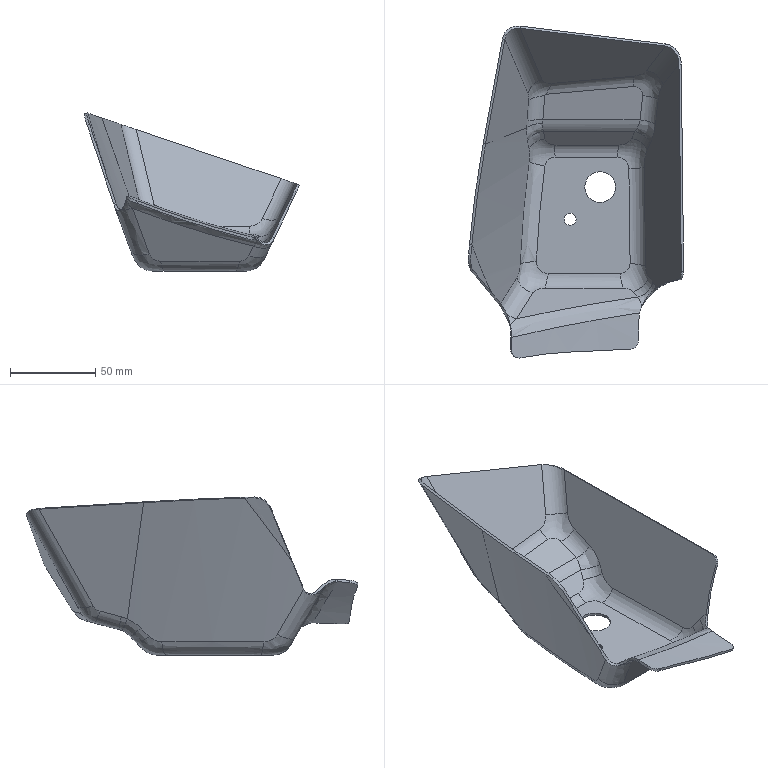Part | 1 solid | 104 faces | box 125.932 x 194.139 x 92.429 mm | volume 51978 mm3 | spline 63 | cylinder 31 | plane 9 | other 1 | commonest cylinder face diameters 20 x10 23 x10 7 x2 18 x2 10 x1 27 x1